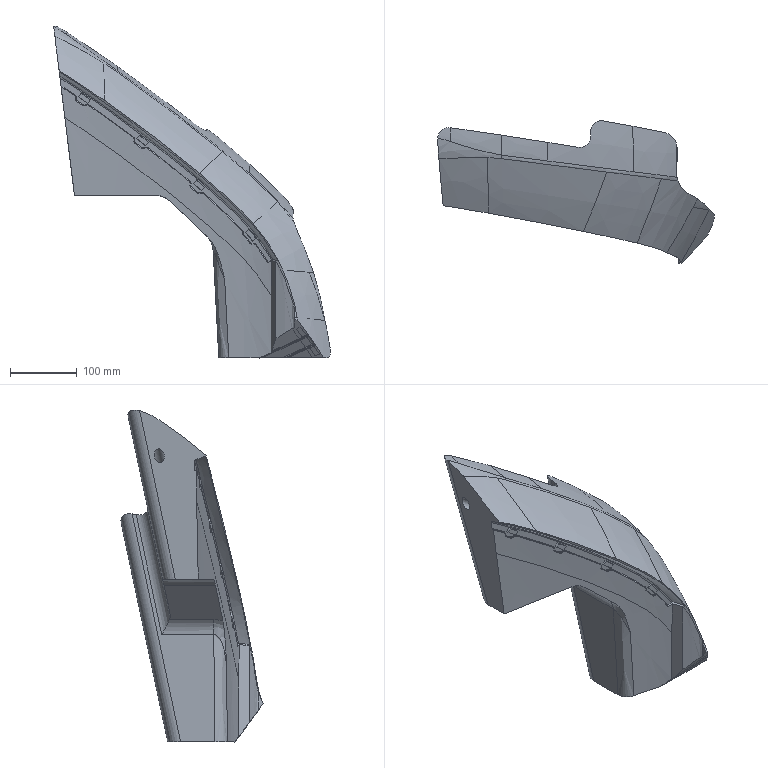Part | STEP file | solid 63 | 1 solid | 196 faces | box 414.488 x 213.171 x 497.487 mm | volume 6813451 mm3 | spline 116 | cylinder 40 | plane 34 | cone 4 | other 2 | commonest cylinder face diameters 6.078 x8 15 x7 38 x7 8.104 x4 10.13 x4 30 x4